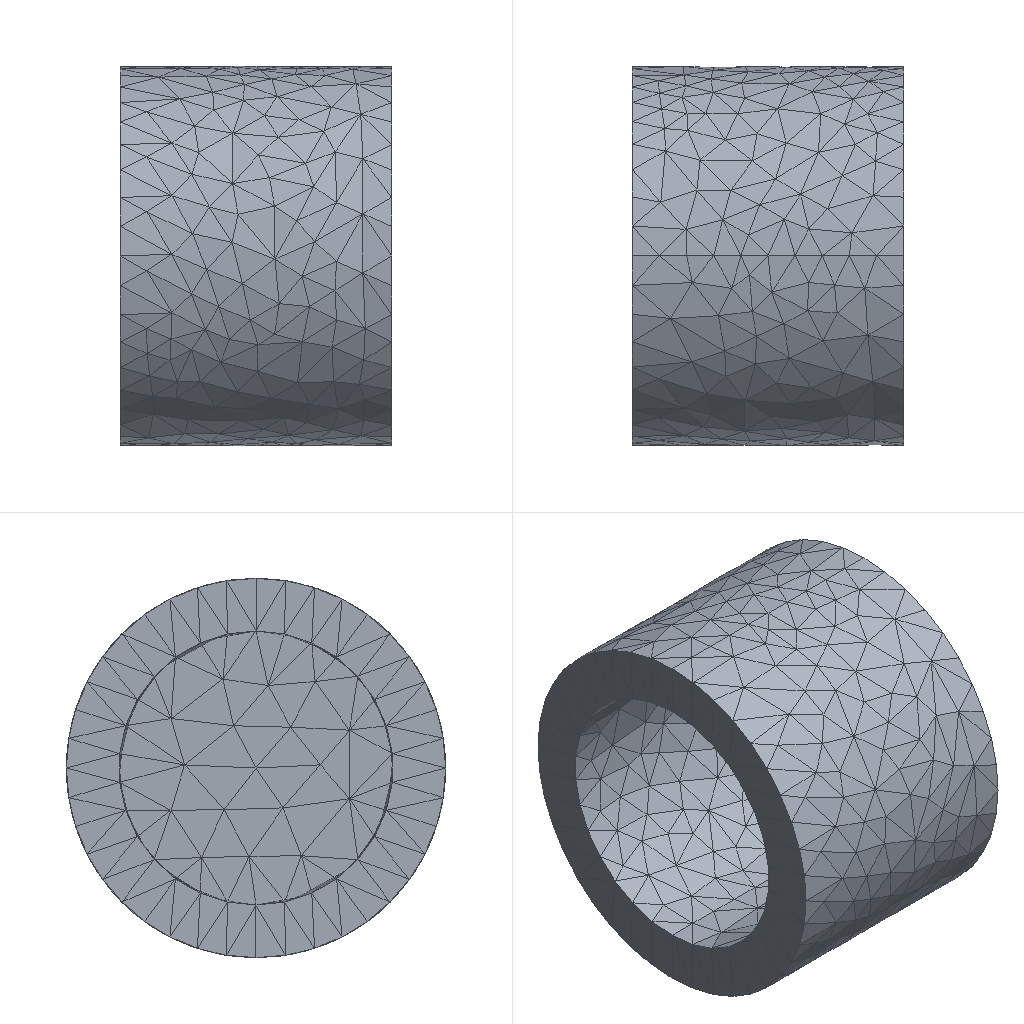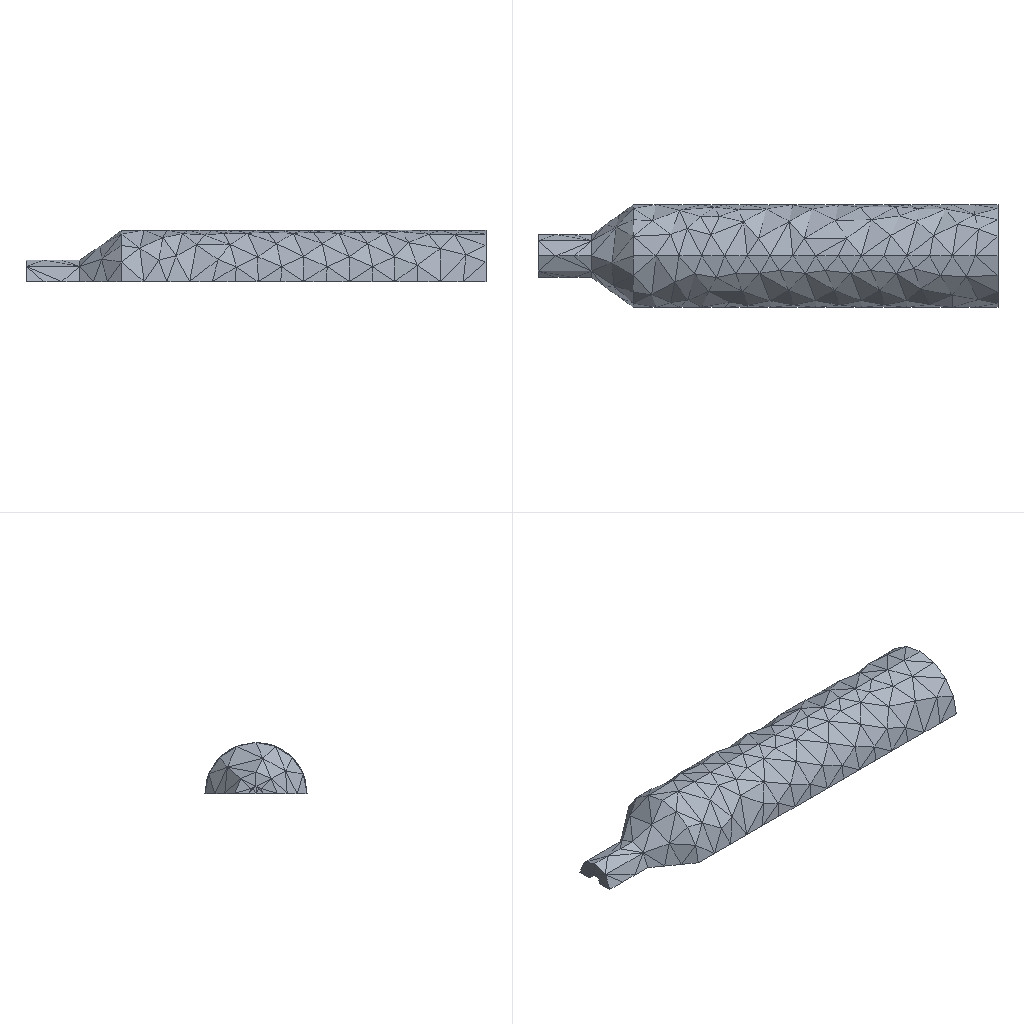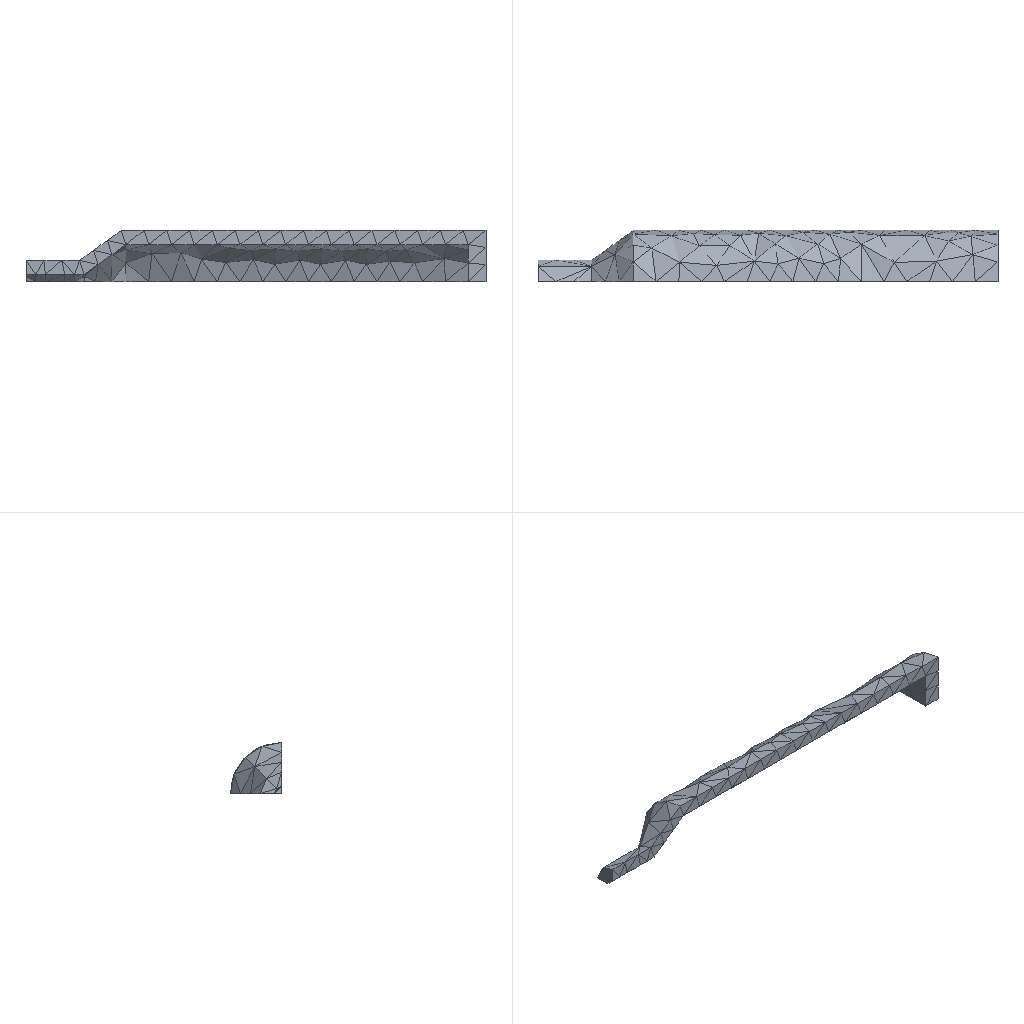Simulation study | ansys workbench
Set-up summary:
category,name,step,type,value,unit,region
solver,ansys_workbench
units,mm-N-s-tonne (MPa),,stated,"/units,MPA"
analysis,deck-1/LS1,,static
load_step,deck-1/LS1,deck-1/LS1,static,nsubst=1; time=1
analysis,deck-2/LS1,,static
load_step,deck-2/LS1,deck-2/LS1,static,nsubst=1; time=1
analysis,deck-3/LS1,,static
load_step,deck-3/LS1,deck-3/LS1,static,nsubst=1; time=1
mesh,deck-1.dat,,nodes,4576
mesh,deck-1.dat,,elements,3452
element_type,SOLID187,,,2524,,deck-1.dat
element_type,SURF154,,,928,,deck-1.dat
mesh,deck-2.dat,,nodes,1584
mesh,deck-2.dat,,elements,1080
element_type,SOLID187,,,716,,deck-2.dat
element_type,SURF154,,,364,,deck-2.dat
mesh,deck-3.dat,,nodes,860
mesh,deck-3.dat,,elements,531
element_type,SOLID187,,,353,,deck-3.dat
element_type,SURF154,,,178,,deck-3.dat
material,Structural Steel,,E,200000,tonne s^-2 mm^-1
material,Structural Steel,,nu,0.3
material,Structural Steel,,density,7.85e-09,tonne mm^-3
material,Structural Steel,,conductivity,60.5,tonne mm s^-3 C^-1
material,Structural Steel,,specific_heat,4.34e+08,mm^2 s^-2 C^-1
material,Structural Steel,,cte,1.2e-05,C^-1
material,Structural Steel,,permeability,10000
material,Structural Steel,,resistivity,0.00017,ohm mm
material,Structural Steel,,E,200000,tonne s^-2 mm^-1
material,Structural Steel,,nu,0.3
material,Structural Steel,,density,7.85e-09,tonne mm^-3
material,Structural Steel,,conductivity,60.5,tonne mm s^-3 C^-1
material,Structural Steel,,specific_heat,4.34e+08,mm^2 s^-2 C^-1
material,Structural Steel,,cte,1.2e-05,C^-1
material,Structural Steel,,permeability,10000
material,Structural Steel,,resistivity,0.00017,ohm mm
material,Structural Steel,,E,200000,tonne s^-2 mm^-1
material,Structural Steel,,nu,0.3
material,Structural Steel,,density,7.85e-09,tonne mm^-3
material,Structural Steel,,conductivity,60.5,tonne mm s^-3 C^-1
material,Structural Steel,,specific_heat,4.34e+08,mm^2 s^-2 C^-1
material,Structural Steel,,cte,1.2e-05,C^-1
material,Structural Steel,,permeability,10000
material,Structural Steel,,resistivity,0.00017,ohm mm
load,"Define Pressure Using Surface Effect Elements ""__""",deck-1/LS1,pressure,20,,SURF154 #2
load,"Define Pressure Using Surface Effect Elements ""__ 2""",deck-1/LS1,pressure,60,,SURF154 #3
load,"Define Pressure Using Surface Effect Elements ""__""",deck-2/LS1,pressure,20,,SURF154 #2
load,"Define Pressure Using Surface Effect Elements ""__ 2""",deck-2/LS1,pressure,60,,SURF154 #3
load,"Define Pressure Using Surface Effect Elements ""__""",deck-3/LS1,pressure,20,,SURF154 #2
load,"Define Pressure Using Surface Effect Elements ""__ 2""",deck-3/LS1,pressure,60,,SURF154 #3
bc,Fixed Supports,deck-1/model,fixed,[dofs=ALL],,_FIXEDSU
bc,Fixed Supports,deck-2/model,fixed,[dofs=ALL],,_FIXEDSU
bc,Fixed Supports,deck-3/model,fixed,[dofs=ALL],,_FIXEDSU
named_set,_FIXEDSU,,node,245
named_set,_FIXEDSU,,node,36
named_set,_FIXEDSU,,node,27
Results summary:
result,analyses[0].index,,,1
result,analyses[0].system,,,SYS
result,analyses[0].deck,,,deck-1.dat
result,analyses[0].solve_status,,,completed
result,analyses[0].analysis_type,,,static
result,analyses[0].physics,,,mechanical
result,analyses[0].unit_system,,,"NMM: mm, ton, N, s, mV, mA, degC"
result,analyses[0].n_sets,,,1
result,analyses[0].load_steps[0].set,set=1,,1
result,analyses[0].load_steps[0].time_or_freq,set=1,,1
result,analyses[0].load_steps[0].max_displacement_magnitude,set=1,,0.07388
result,analyses[0].load_steps[0].max_von_mises_nodal,set=1,,160.095
result,analyses[0].load_steps[0].reaction_force_sum_xyz[1],set=1,,-2.62844e-09
result,analyses[0].load_steps[0].reaction_force_sum_xyz[2],set=1,,-8.86985e-10
result,analyses[0].load_steps[0].reaction_force_sum_xyz[3],set=1,,1.36911e-08
result,analyses[1].index,,,2
result,analyses[1].system,,,SYS-1
result,analyses[1].deck,,,deck-2.dat
result,analyses[1].solve_status,,,completed
result,analyses[1].analysis_type,,,static
result,analyses[1].physics,,,mechanical
result,analyses[1].unit_system,,,"NMM: mm, ton, N, s, mV, mA, degC"
result,analyses[1].n_sets,,,1
result,analyses[1].load_steps[0].set,set=1,,1
result,analyses[1].load_steps[0].time_or_freq,set=1,,1
result,analyses[1].load_steps[0].max_displacement_magnitude,set=1,,240.067
result,analyses[1].load_steps[0].max_von_mises_nodal,set=1,,9767.61
result,analyses[1].load_steps[0].reaction_force_sum_xyz[1],set=1,,-3.33099e-05
result,analyses[1].load_steps[0].reaction_force_sum_xyz[2],set=1,,7.42398e-06
result,analyses[1].load_steps[0].reaction_force_sum_xyz[3],set=1,,-6.1611e+06
result,analyses[2].index,,,3
result,analyses[2].system,,,SYS-2
result,analyses[2].deck,,,deck-3.dat
result,analyses[2].solve_status,,,completed
result,analyses[2].analysis_type,,,static
result,analyses[2].physics,,,mechanical
result,analyses[2].unit_system,,,"NMM: mm, ton, N, s, mV, mA, degC"
result,analyses[2].n_sets,,,1
result,analyses[2].load_steps[0].set,set=1,,1
result,analyses[2].load_steps[0].time_or_freq,set=1,,1
result,analyses[2].load_steps[0].max_displacement_magnitude,set=1,,2111.88
result,analyses[2].load_steps[0].max_von_mises_nodal,set=1,,40134.4
result,analyses[2].load_steps[0].reaction_force_sum_xyz[1],set=1,,-0.000558
result,analyses[2].load_steps[0].reaction_force_sum_xyz[2],set=1,,-3.08055e+06
result,analyses[2].load_steps[0].reaction_force_sum_xyz[3],set=1,,-3.08055e+06